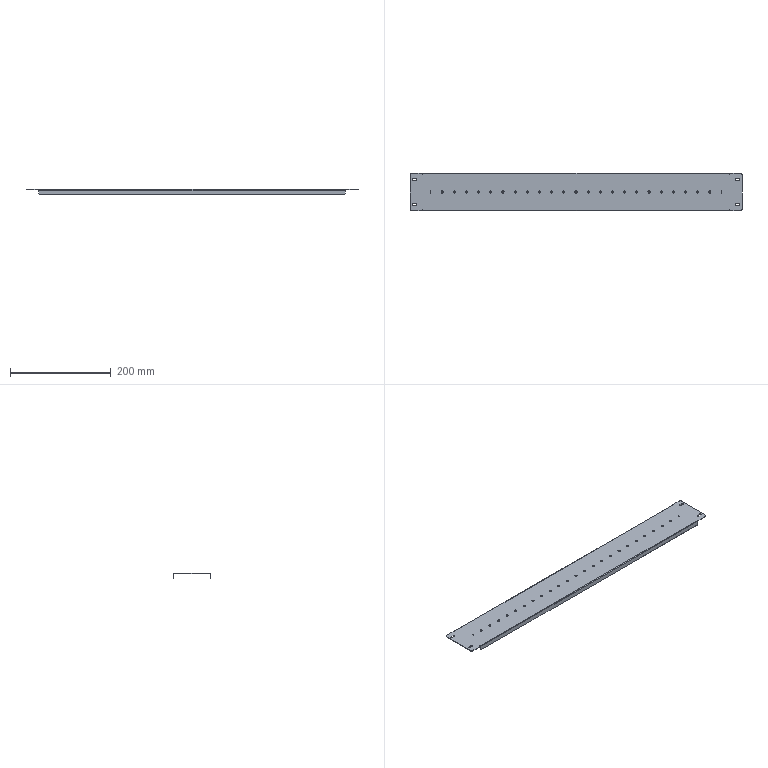Part | SolidWorks | features ICE 2, MirrorPattern 2, SMBaseFlange 2, EdgeFlange 1, Fillet 1, FlatPattern 1, SheetMetal 1 | 1 solid | 117 faces | box 660 x 74 x 10 mm | volume 58966 mm3 | cylinder 73 | plane 44 | commonest cylinder face diameters 4.2 x61 6 x8 0.4 x2 2.4 x2